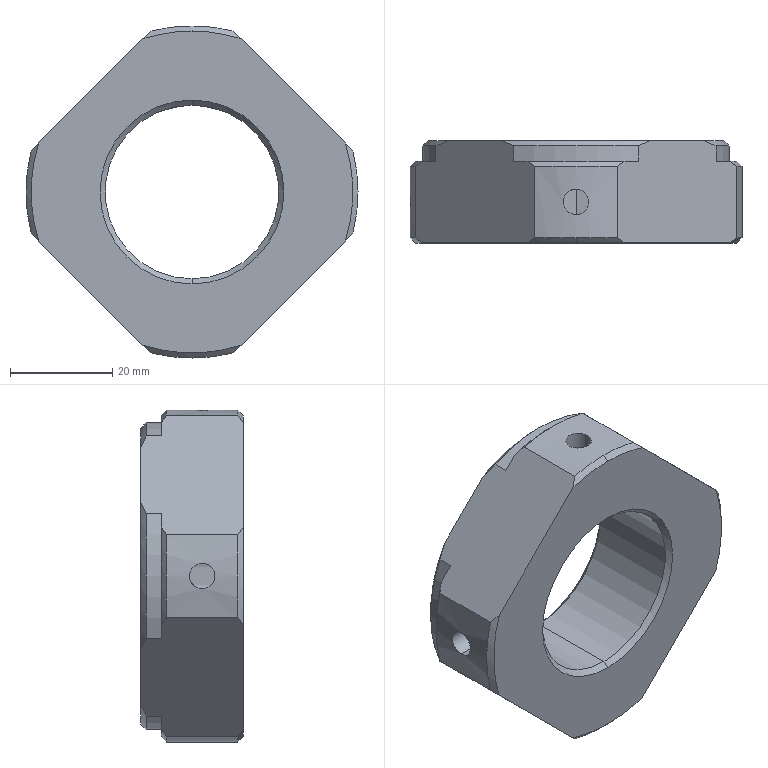Part | STEP file | 10-20 lock nut | 1 solid | 45 faces | box 65 x 20 x 65 mm | volume 38511 mm3 | cone 19 | cylinder 16 | plane 10 | commonest cylinder face diameters 60 x5 65 x5 5 x4 34 x2